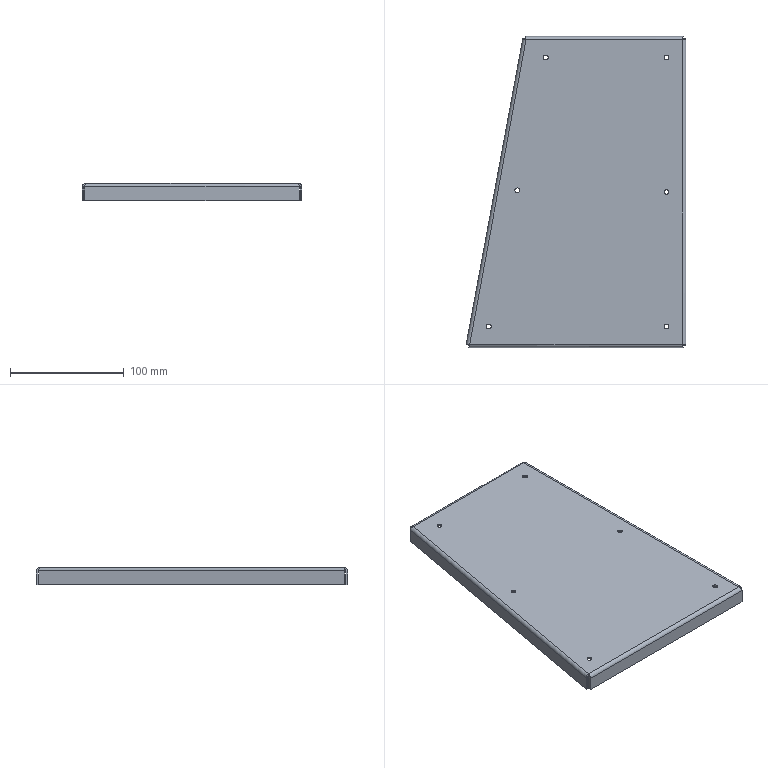Part | STEP file | Drive box door QY-1-38 | 1 solid | 50 faces | box 192.833 x 273 x 15 mm | volume 84976 mm3 | plane 22 | cylinder 20 | spline 8 | commonest cylinder face diameters 4.2 x12 3 x4 6 x4